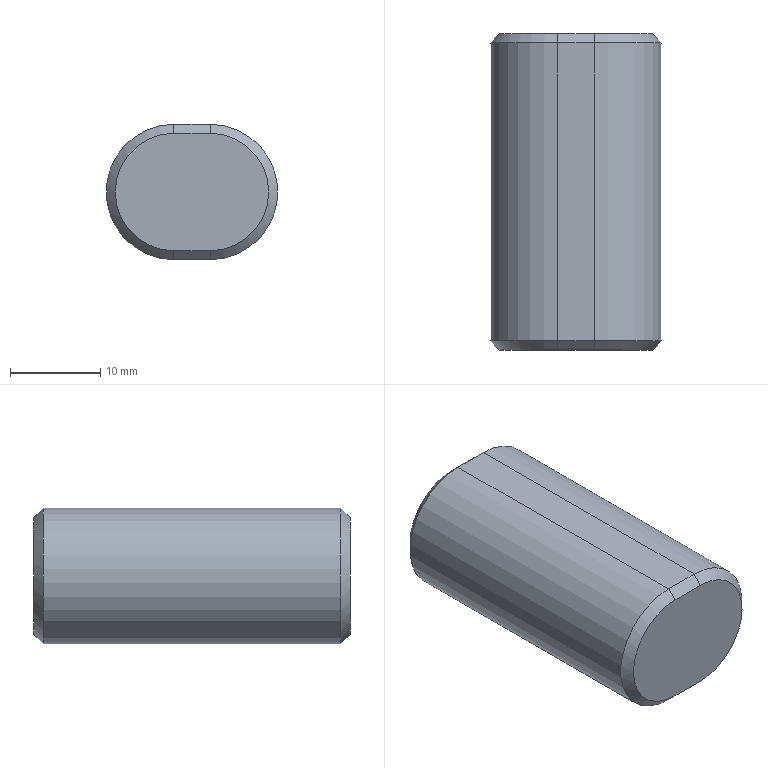Part | SolidWorks | features Chamfer 1, Extrusion 1 | 1 solid | 14 faces | box 19 x 35 x 15 mm | volume 8232 mm3 | plane 8 | cone 4 | cylinder 2 | commonest cylinder face diameters 15 x2
STEP:
#1=CARTESIAN_POINT('',(-2.,34.,-7.5));
#2=VERTEX_POINT('',#1);
#3=CARTESIAN_POINT('',(-2.,1.,-7.5));
#4=VERTEX_POINT('',#3);
#5=CARTESIAN_POINT('',(-2.,35.,-7.5));
#6=DIRECTION('',(0.,-1.,0.));
#7=VECTOR('',#6,1000.);
#8=LINE('',#5,#7);
#9=EDGE_CURVE('',#2,#4,#8,.T.);
#10=ORIENTED_EDGE('',*,*,#9,.T.);
#11=CARTESIAN_POINT('',(-2.,1.,7.5));
#12=VERTEX_POINT('',#11);
#13=CARTESIAN_POINT('',(-2.,1.,0.));
#14=DIRECTION('',(0.,1.,0.));
#15=DIRECTION('',(0.,0.,1.));
#16=AXIS2_PLACEMENT_3D('',#13,#14,#15);
#17=CIRCLE('',#16,7.5);
#18=EDGE_CURVE('',#4,#12,#17,.T.);
#19=ORIENTED_EDGE('',*,*,#18,.T.);
#20=CARTESIAN_POINT('',(-2.,34.,7.5));
#21=VERTEX_POINT('',#20);
#22=CARTESIAN_POINT('',(-2.,35.,7.5));
#23=DIRECTION('',(0.,-1.,0.));
#24=VECTOR('',#23,1000.);
#25=LINE('',#22,#24);
#26=EDGE_CURVE('',#21,#12,#25,.T.);
#27=ORIENTED_EDGE('',*,*,#26,.F.);
#28=CARTESIAN_POINT('',(-2.,34.,0.));
#29=DIRECTION('',(0.,-1.,0.));
#30=DIRECTION('',(0.,0.,1.));
#31=AXIS2_PLACEMENT_3D('',#28,#29,#30);
#32=CIRCLE('',#31,7.5);
#33=EDGE_CURVE('',#21,#2,#32,.T.);
#34=ORIENTED_EDGE('',*,*,#33,.T.);
#35=EDGE_LOOP('',(#10,#19,#27,#34));
#36=FACE_OUTER_BOUND('',#35,.T.);
#37=CARTESIAN_POINT('',(-2.,35.,0.));
#38=DIRECTION('',(0.,-1.,0.));
#39=DIRECTION('',(0.,0.,-1.));
#40=AXIS2_PLACEMENT_3D('',#37,#38,#39);
#41=CYLINDRICAL_SURFACE('',#40,7.5);
#42=ADVANCED_FACE('',(#36),#41,.T.);
#43=ORIENTED_EDGE('',*,*,#26,.T.);
#44=CARTESIAN_POINT('',(2.,1.,7.5));
#45=VERTEX_POINT('',#44);
#46=CARTESIAN_POINT('',(-2.,1.,7.5));
#47=DIRECTION('',(1.,0.,0.));
#48=VECTOR('',#47,1000.);
#49=LINE('',#46,#48);
#50=EDGE_CURVE('',#12,#45,#49,.T.);
#51=ORIENTED_EDGE('',*,*,#50,.T.);
#52=CARTESIAN_POINT('',(2.,34.,7.5));
#53=VERTEX_POINT('',#52);
#54=CARTESIAN_POINT('',(2.,35.,7.5));
#55=DIRECTION('',(0.,-1.,0.));
#56=VECTOR('',#55,1000.);
#57=LINE('',#54,#56);
#58=EDGE_CURVE('',#53,#45,#57,.T.);
#59=ORIENTED_EDGE('',*,*,#58,.F.);
#60=CARTESIAN_POINT('',(-2.,34.,7.5));
#61=DIRECTION('',(-1.,0.,0.));
#62=VECTOR('',#61,1000.);
#63=LINE('',#60,#62);
#64=EDGE_CURVE('',#53,#21,#63,.T.);
#65=ORIENTED_EDGE('',*,*,#64,.T.);
#66=EDGE_LOOP('',(#43,#51,#59,#65));
#67=FACE_OUTER_BOUND('',#66,.T.);
#68=CARTESIAN_POINT('',(-2.,35.,7.5));
#69=DIRECTION('',(0.,0.,-1.));
#70=DIRECTION('',(-1.,0.,0.));
#71=AXIS2_PLACEMENT_3D('',#68,#69,#70);
#72=PLANE('',#71);
#73=ADVANCED_FACE('',(#67),#72,.F.);
#74=ORIENTED_EDGE('',*,*,#58,.T.);
#75=CARTESIAN_POINT('',(2.,1.,-7.5));
#76=VERTEX_POINT('',#75);
#77=CARTESIAN_POINT('',(2.,1.,0.));
#78=DIRECTION('',(0.,1.,0.));
#79=DIRECTION('',(0.,0.,1.));
#80=AXIS2_PLACEMENT_3D('',#77,#78,#79);
#81=CIRCLE('',#80,7.5);
#82=EDGE_CURVE('',#45,#76,#81,.T.);
#83=ORIENTED_EDGE('',*,*,#82,.T.);
#84=CARTESIAN_POINT('',(2.,34.,-7.5));
#85=VERTEX_POINT('',#84);
#86=CARTESIAN_POINT('',(2.,35.,-7.5));
#87=DIRECTION('',(0.,-1.,0.));
#88=VECTOR('',#87,1000.);
#89=LINE('',#86,#88);
#90=EDGE_CURVE('',#85,#76,#89,.T.);
#91=ORIENTED_EDGE('',*,*,#90,.F.);
#92=CARTESIAN_POINT('',(2.,34.,0.));
#93=DIRECTION('',(0.,-1.,0.));
#94=DIRECTION('',(0.,0.,1.));
#95=AXIS2_PLACEMENT_3D('',#92,#93,#94);
#96=CIRCLE('',#95,7.5);
#97=EDGE_CURVE('',#85,#53,#96,.T.);
#98=ORIENTED_EDGE('',*,*,#97,.T.);
#99=EDGE_LOOP('',(#74,#83,#91,#98));
#100=FACE_OUTER_BOUND('',#99,.T.);
#101=CARTESIAN_POINT('',(2.,35.,0.));
#102=DIRECTION('',(0.,-1.,0.));
#103=DIRECTION('',(0.,0.,-1.));
#104=AXIS2_PLACEMENT_3D('',#101,#102,#103);
#105=CYLINDRICAL_SURFACE('',#104,7.5);
#106=ADVANCED_FACE('',(#100),#105,.T.);
#107=ORIENTED_EDGE('',*,*,#90,.T.);
#108=CARTESIAN_POINT('',(-2.,1.,-7.5));
#109=DIRECTION('',(-1.,0.,0.));
#110=VECTOR('',#109,1000.);
#111=LINE('',#108,#110);
#112=EDGE_CURVE('',#76,#4,#111,.T.);
#113=ORIENTED_EDGE('',*,*,#112,.T.);
#114=ORIENTED_EDGE('',*,*,#9,.F.);
#115=CARTESIAN_POINT('',(2.,34.,-7.5));
#116=DIRECTION('',(1.,0.,0.));
#117=VECTOR('',#116,1000.);
#118=LINE('',#115,#117);
#119=EDGE_CURVE('',#2,#85,#118,.T.);
#120=ORIENTED_EDGE('',*,*,#119,.T.);
#121=EDGE_LOOP('',(#107,#113,#114,#120));
#122=FACE_OUTER_BOUND('',#121,.T.);
#123=CARTESIAN_POINT('',(-2.,35.,-7.5));
#124=DIRECTION('',(0.,0.,1.));
#125=DIRECTION('',(1.,0.,0.));
#126=AXIS2_PLACEMENT_3D('',#123,#124,#125);
#127=PLANE('',#126);
#128=ADVANCED_FACE('',(#122),#127,.F.);
#129=CARTESIAN_POINT('',(-2.,35.,6.5));
#130=VERTEX_POINT('',#129);
#131=CARTESIAN_POINT('',(2.,35.,6.5));
#132=VERTEX_POINT('',#131);
#133=CARTESIAN_POINT('',(2.,35.,6.5));
#134=DIRECTION('',(1.,0.,0.));
#135=VECTOR('',#134,1000.);
#136=LINE('',#133,#135);
#137=EDGE_CURVE('',#130,#132,#136,.T.);
#138=ORIENTED_EDGE('',*,*,#137,.T.);
#139=CARTESIAN_POINT('',(2.,35.,-6.5));
#140=VERTEX_POINT('',#139);
#141=CARTESIAN_POINT('',(2.,35.,0.));
#142=DIRECTION('',(0.,1.,0.));
#143=DIRECTION('',(0.,0.,1.));
#144=AXIS2_PLACEMENT_3D('',#141,#142,#143);
#145=CIRCLE('',#144,6.5);
#146=EDGE_CURVE('',#132,#140,#145,.T.);
#147=ORIENTED_EDGE('',*,*,#146,.T.);
#148=CARTESIAN_POINT('',(-2.,35.,-6.5));
#149=VERTEX_POINT('',#148);
#150=CARTESIAN_POINT('',(-2.,35.,-6.5));
#151=DIRECTION('',(-1.,0.,0.));
#152=VECTOR('',#151,1000.);
#153=LINE('',#150,#152);
#154=EDGE_CURVE('',#140,#149,#153,.T.);
#155=ORIENTED_EDGE('',*,*,#154,.T.);
#156=CARTESIAN_POINT('',(-2.,35.,0.));
#157=DIRECTION('',(0.,1.,0.));
#158=DIRECTION('',(0.,0.,1.));
#159=AXIS2_PLACEMENT_3D('',#156,#157,#158);
#160=CIRCLE('',#159,6.5);
#161=EDGE_CURVE('',#149,#130,#160,.T.);
#162=ORIENTED_EDGE('',*,*,#161,.T.);
#163=EDGE_LOOP('',(#138,#147,#155,#162));
#164=FACE_OUTER_BOUND('',#163,.T.);
#165=CARTESIAN_POINT('',(-2.,35.,0.));
#166=DIRECTION('',(0.,1.,0.));
#167=DIRECTION('',(0.,0.,1.));
#168=AXIS2_PLACEMENT_3D('',#165,#166,#167);
#169=PLANE('',#168);
#170=ADVANCED_FACE('',(#164),#169,.T.);
#171=CARTESIAN_POINT('',(-2.,0.,-6.5));
#172=VERTEX_POINT('',#171);
#173=CARTESIAN_POINT('',(2.,0.,-6.5));
#174=VERTEX_POINT('',#173);
#175=CARTESIAN_POINT('',(-2.,0.,-6.5));
#176=DIRECTION('',(1.,0.,0.));
#177=VECTOR('',#176,1000.);
#178=LINE('',#175,#177);
#179=EDGE_CURVE('',#172,#174,#178,.T.);
#180=ORIENTED_EDGE('',*,*,#179,.T.);
#181=CARTESIAN_POINT('',(2.,0.,6.5));
#182=VERTEX_POINT('',#181);
#183=CARTESIAN_POINT('',(2.,0.,0.));
#184=DIRECTION('',(0.,-1.,0.));
#185=DIRECTION('',(0.,0.,1.));
#186=AXIS2_PLACEMENT_3D('',#183,#184,#185);
#187=CIRCLE('',#186,6.5);
#188=EDGE_CURVE('',#174,#182,#187,.T.);
#189=ORIENTED_EDGE('',*,*,#188,.T.);
#190=CARTESIAN_POINT('',(-2.,0.,6.5));
#191=VERTEX_POINT('',#190);
#192=CARTESIAN_POINT('',(-2.,0.,6.5));
#193=DIRECTION('',(-1.,0.,0.));
#194=VECTOR('',#193,1000.);
#195=LINE('',#192,#194);
#196=EDGE_CURVE('',#182,#191,#195,.T.);
#197=ORIENTED_EDGE('',*,*,#196,.T.);
#198=CARTESIAN_POINT('',(-2.,0.,0.));
#199=DIRECTION('',(0.,-1.,0.));
#200=DIRECTION('',(0.,0.,1.));
#201=AXIS2_PLACEMENT_3D('',#198,#199,#200);
#202=CIRCLE('',#201,6.5);
#203=EDGE_CURVE('',#191,#172,#202,.T.);
#204=ORIENTED_EDGE('',*,*,#203,.T.);
#205=EDGE_LOOP('',(#180,#189,#197,#204));
#206=FACE_OUTER_BOUND('',#205,.T.);
#207=CARTESIAN_POINT('',(-2.,0.,0.));
#208=DIRECTION('',(0.,1.,0.));
#209=DIRECTION('',(0.,0.,1.));
#210=AXIS2_PLACEMENT_3D('',#207,#208,#209);
#211=PLANE('',#210);
#212=ADVANCED_FACE('',(#206),#211,.F.);
#213=CARTESIAN_POINT('',(-2.,0.,-6.5));
#214=DIRECTION('',(0.,0.7071,-0.7071));
#215=VECTOR('',#214,1000.);
#216=LINE('',#213,#215);
#217=EDGE_CURVE('',#172,#4,#216,.T.);
#218=ORIENTED_EDGE('',*,*,#217,.F.);
#219=ORIENTED_EDGE('',*,*,#203,.F.);
#220=CARTESIAN_POINT('',(-2.,1.,7.5));
#221=DIRECTION('',(0.,-0.7071,-0.7071));
#222=VECTOR('',#221,1000.);
#223=LINE('',#220,#222);
#224=EDGE_CURVE('',#12,#191,#223,.T.);
#225=ORIENTED_EDGE('',*,*,#224,.F.);
#226=ORIENTED_EDGE('',*,*,#18,.F.);
#227=EDGE_LOOP('',(#218,#219,#225,#226));
#228=FACE_OUTER_BOUND('',#227,.T.);
#229=CARTESIAN_POINT('',(-2.,1.,0.));
#230=DIRECTION('',(0.,1.,0.));
#231=DIRECTION('',(0.,0.,1.));
#232=AXIS2_PLACEMENT_3D('',#229,#230,#231);
#233=CONICAL_SURFACE('',#232,7.5,0.7854);
#234=ADVANCED_FACE('',(#228),#233,.T.);
#235=ORIENTED_EDGE('',*,*,#224,.T.);
#236=ORIENTED_EDGE('',*,*,#196,.F.);
#237=CARTESIAN_POINT('',(2.,1.,7.5));
#238=DIRECTION('',(0.,-0.7071,-0.7071));
#239=VECTOR('',#238,1000.);
#240=LINE('',#237,#239);
#241=EDGE_CURVE('',#45,#182,#240,.T.);
#242=ORIENTED_EDGE('',*,*,#241,.F.);
#243=ORIENTED_EDGE('',*,*,#50,.F.);
#244=EDGE_LOOP('',(#235,#236,#242,#243));
#245=FACE_OUTER_BOUND('',#244,.T.);
#246=CARTESIAN_POINT('',(-2.,1.,7.5));
#247=DIRECTION('',(0.,0.7071,-0.7071));
#248=DIRECTION('',(1.,0.,0.));
#249=AXIS2_PLACEMENT_3D('',#246,#247,#248);
#250=PLANE('',#249);
#251=ADVANCED_FACE('',(#245),#250,.F.);
#252=ORIENTED_EDGE('',*,*,#217,.T.);
#253=ORIENTED_EDGE('',*,*,#112,.F.);
#254=CARTESIAN_POINT('',(2.,0.,-6.5));
#255=DIRECTION('',(0.,0.7071,-0.7071));
#256=VECTOR('',#255,1000.);
#257=LINE('',#254,#256);
#258=EDGE_CURVE('',#174,#76,#257,.T.);
#259=ORIENTED_EDGE('',*,*,#258,.F.);
#260=ORIENTED_EDGE('',*,*,#179,.F.);
#261=EDGE_LOOP('',(#252,#253,#259,#260));
#262=FACE_OUTER_BOUND('',#261,.T.);
#263=CARTESIAN_POINT('',(-2.,1.,-7.5));
#264=DIRECTION('',(0.,0.7071,0.7071));
#265=DIRECTION('',(-1.,0.,0.));
#266=AXIS2_PLACEMENT_3D('',#263,#264,#265);
#267=PLANE('',#266);
#268=ADVANCED_FACE('',(#262),#267,.F.);
#269=ORIENTED_EDGE('',*,*,#241,.T.);
#270=ORIENTED_EDGE('',*,*,#188,.F.);
#271=ORIENTED_EDGE('',*,*,#258,.T.);
#272=ORIENTED_EDGE('',*,*,#82,.F.);
#273=EDGE_LOOP('',(#269,#270,#271,#272));
#274=FACE_OUTER_BOUND('',#273,.T.);
#275=CARTESIAN_POINT('',(2.,1.,0.));
#276=DIRECTION('',(0.,1.,0.));
#277=DIRECTION('',(0.,0.,1.));
#278=AXIS2_PLACEMENT_3D('',#275,#276,#277);
#279=CONICAL_SURFACE('',#278,7.5,0.7854);
#280=ADVANCED_FACE('',(#274),#279,.T.);
#281=CARTESIAN_POINT('',(-2.,34.,-7.5));
#282=DIRECTION('',(0.,0.7071,0.7071));
#283=VECTOR('',#282,1000.);
#284=LINE('',#281,#283);
#285=EDGE_CURVE('',#2,#149,#284,.T.);
#286=ORIENTED_EDGE('',*,*,#285,.F.);
#287=ORIENTED_EDGE('',*,*,#33,.F.);
#288=CARTESIAN_POINT('',(-2.,35.,6.5));
#289=DIRECTION('',(0.,-0.7071,0.7071));
#290=VECTOR('',#289,1000.);
#291=LINE('',#288,#290);
#292=EDGE_CURVE('',#130,#21,#291,.T.);
#293=ORIENTED_EDGE('',*,*,#292,.F.);
#294=ORIENTED_EDGE('',*,*,#161,.F.);
#295=EDGE_LOOP('',(#286,#287,#293,#294));
#296=FACE_OUTER_BOUND('',#295,.T.);
#297=CARTESIAN_POINT('',(-2.,35.,0.));
#298=DIRECTION('',(0.,-1.,0.));
#299=DIRECTION('',(0.,0.,-1.));
#300=AXIS2_PLACEMENT_3D('',#297,#298,#299);
#301=CONICAL_SURFACE('',#300,6.5,0.7854);
#302=ADVANCED_FACE('',(#296),#301,.T.);
#303=ORIENTED_EDGE('',*,*,#292,.T.);
#304=ORIENTED_EDGE('',*,*,#64,.F.);
#305=CARTESIAN_POINT('',(2.,35.,6.5));
#306=DIRECTION('',(0.,-0.7071,0.7071));
#307=VECTOR('',#306,1000.);
#308=LINE('',#305,#307);
#309=EDGE_CURVE('',#132,#53,#308,.T.);
#310=ORIENTED_EDGE('',*,*,#309,.F.);
#311=ORIENTED_EDGE('',*,*,#137,.F.);
#312=EDGE_LOOP('',(#303,#304,#310,#311));
#313=FACE_OUTER_BOUND('',#312,.T.);
#314=CARTESIAN_POINT('',(-2.,35.,6.5));
#315=DIRECTION('',(0.,0.7071,0.7071));
#316=DIRECTION('',(-1.,0.,0.));
#317=AXIS2_PLACEMENT_3D('',#314,#315,#316);
#318=PLANE('',#317);
#319=ADVANCED_FACE('',(#313),#318,.T.);
#320=ORIENTED_EDGE('',*,*,#285,.T.);
#321=ORIENTED_EDGE('',*,*,#154,.F.);
#322=CARTESIAN_POINT('',(2.,34.,-7.5));
#323=DIRECTION('',(0.,0.7071,0.7071));
#324=VECTOR('',#323,1000.);
#325=LINE('',#322,#324);
#326=EDGE_CURVE('',#85,#140,#325,.T.);
#327=ORIENTED_EDGE('',*,*,#326,.F.);
#328=ORIENTED_EDGE('',*,*,#119,.F.);
#329=EDGE_LOOP('',(#320,#321,#327,#328));
#330=FACE_OUTER_BOUND('',#329,.T.);
#331=CARTESIAN_POINT('',(-2.,35.,-6.5));
#332=DIRECTION('',(0.,0.7071,-0.7071));
#333=DIRECTION('',(1.,0.,0.));
#334=AXIS2_PLACEMENT_3D('',#331,#332,#333);
#335=PLANE('',#334);
#336=ADVANCED_FACE('',(#330),#335,.T.);
#337=ORIENTED_EDGE('',*,*,#309,.T.);
#338=ORIENTED_EDGE('',*,*,#97,.F.);
#339=ORIENTED_EDGE('',*,*,#326,.T.);
#340=ORIENTED_EDGE('',*,*,#146,.F.);
#341=EDGE_LOOP('',(#337,#338,#339,#340));
#342=FACE_OUTER_BOUND('',#341,.T.);
#343=CARTESIAN_POINT('',(2.,35.,0.));
#344=DIRECTION('',(0.,-1.,0.));
#345=DIRECTION('',(0.,0.,-1.));
#346=AXIS2_PLACEMENT_3D('',#343,#344,#345);
#347=CONICAL_SURFACE('',#346,6.5,0.7854);
#348=ADVANCED_FACE('',(#342),#347,.T.);
#349=CLOSED_SHELL('',(#42,#73,#106,#128,#170,#212,#234,#251,#268,#280,#302,#319,#336,#348));
#350=MANIFOLD_SOLID_BREP('',#349);
#351=CARTESIAN_POINT('',(0.,0.,0.));
#352=DIRECTION('',(0.,0.,1.));
#353=DIRECTION('',(1.,0.,0.));
#354=AXIS2_PLACEMENT_3D('',#351,#352,#353);
#355=(LENGTH_UNIT()NAMED_UNIT(*)SI_UNIT(.MILLI.,.METRE.));
#356=UNCERTAINTY_MEASURE_WITH_UNIT(LENGTH_MEASURE(0.00001),#355,'','');
#357=(NAMED_UNIT(*)PLANE_ANGLE_UNIT()SI_UNIT($,.RADIAN.));
#358=(NAMED_UNIT(*)SI_UNIT($,.STERADIAN.)SOLID_ANGLE_UNIT());
#359=(GEOMETRIC_REPRESENTATION_CONTEXT(3)GLOBAL_UNCERTAINTY_ASSIGNED_CONTEXT((#356))GLOBAL_UNIT_ASSIGNED_CONTEXT((#355,#357,#358))REPRESENTATION_CONTEXT('',''));
#360=ADVANCED_BREP_SHAPE_REPRESENTATION('',(#350,#354),#359);